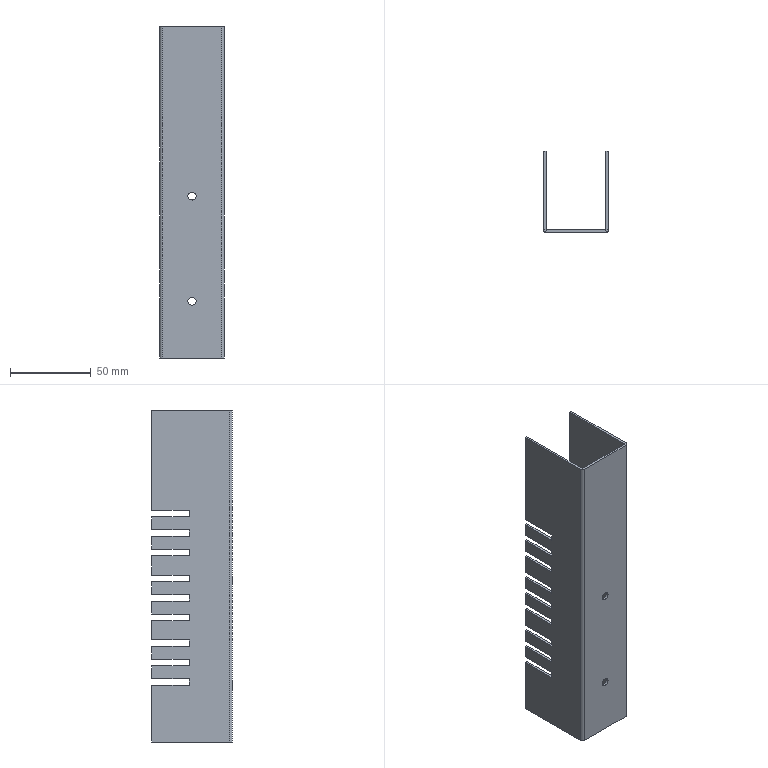Part | SolidWorks | features MoveFace 2, Cut 1, FlatPattern 1, ICE 1, LPattern 1, SMBaseFlange 1, SheetMetal 1 | 1 solid | 98 faces | box 40 x 50 x 205 mm | volume 39291 mm3 | plane 90 | cylinder 8 | commonest cylinder face diameters 5 x4 0.4 x2 3.4 x2